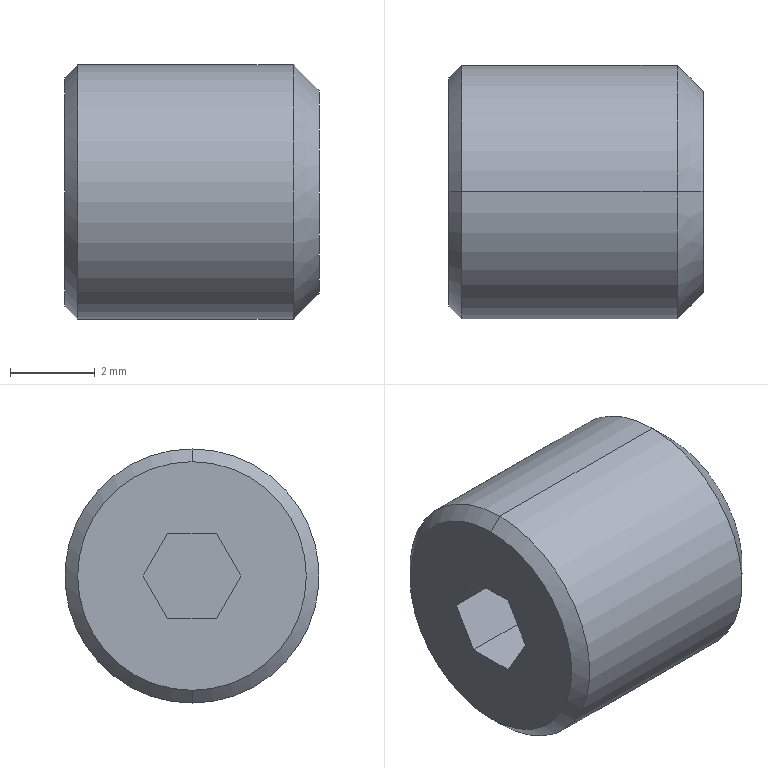Part | SolidWorks | features BaseBody 1 | 1 solid | 16 faces | box 6 x 6 x 6 mm | volume 154.933 mm3 | plane 8 | cone 6 | cylinder 2 | commonest cylinder face diameters 6 x2